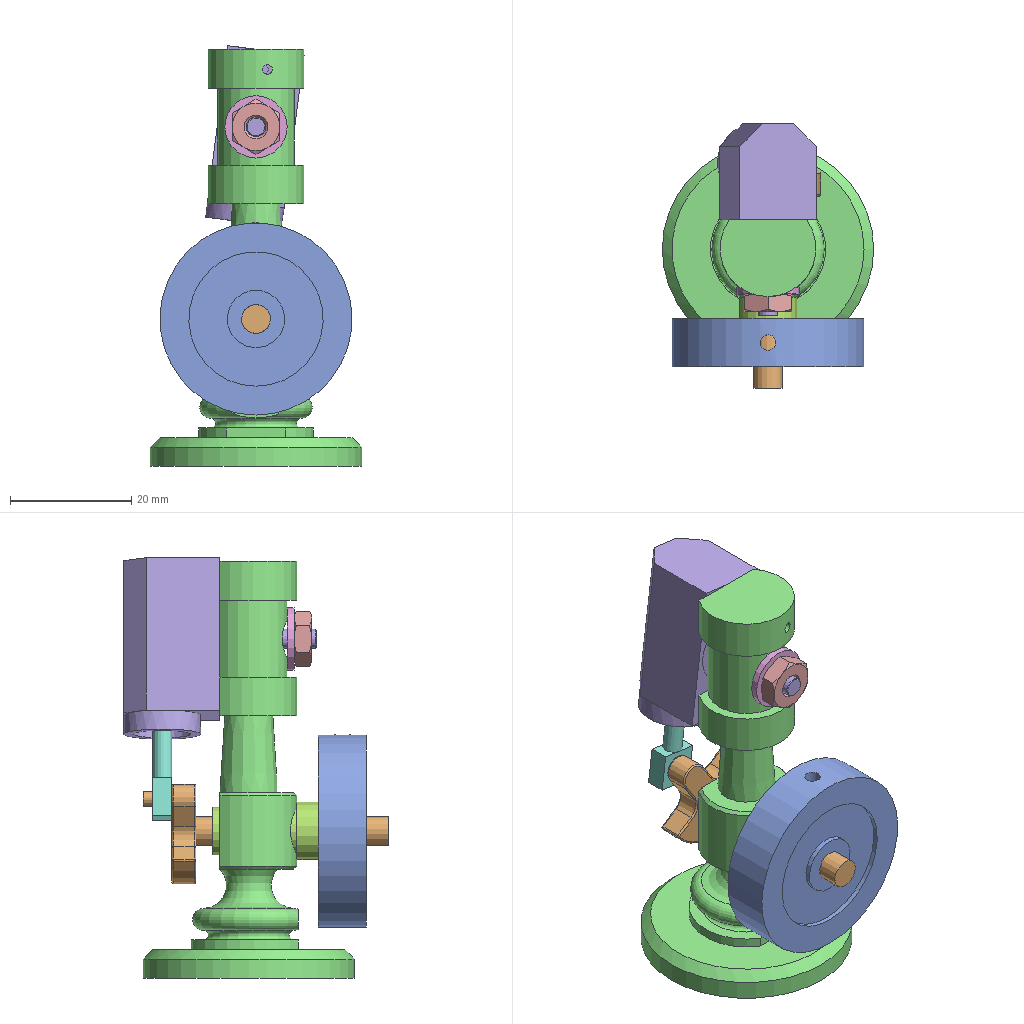Assembly | NX | 8 different items | 8 placed | box 35 x 44 x 70 mm
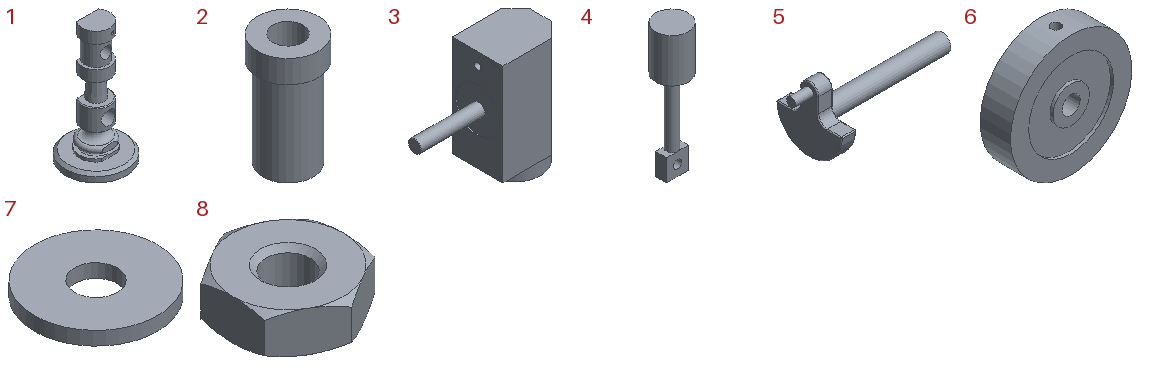Parts list (item | quantity | size | volume | features):
1 | x1 | 34.925 x 34.925 x 68.955 mm | 12101 mm3 | features DATUM_CSYS 9, SKETCH 8, EXTRUDE 5, CYLINDER 4, SWP104 3, CHAMFER 2, Intersection Curve 2, CPROJ 1
2 | x1 | 9.525 x 9.525 x 17.463 mm | 630.793 mm3 | features DATUM_CSYS 2, SKETCH 1, SWP104 1
3 | x1 | 31.75 x 12.7 x 28.575 mm | 3399 mm3 | features DATUM_CSYS 7, SKETCH 6, EXTRUDE 4, CYLINDER 2, CHAMFER 1, SWP104 1
4 | x1 | 9.525 x 9.525 x 38.1 mm | 1170 mm3 | features DATUM_CSYS 4, SKETCH 3, EXTRUDE 2, SWP104 1
5 | x1 | 40.481 x 17.455 x 17.462 mm | 1225 mm3 | features DATUM_CSYS 4, EXTRUDE 3, SKETCH 3, BLEND 1
6 | x1 | 31.75 x 7.938 x 31.75 mm | 5557 mm3 | features DATUM_CSYS 3, CYLINDER 2, SKETCH 2, DATUM_PLANE 1, SWP104 1
7 | x1 | 10.312 x 10.312 x 1.143 mm | 83.953 mm3 | features DATUM_CSYS 2, EXTRUDE 1, SKETCH 1
8 | x1 | 7.925 x 9.151 x 2.896 mm | 131.895 mm3 | features DATUM_CSYS 4, EXTRACT_DATUM_AXIS 4, SKETCH 3, EXTRACT_DATUM_PLANE 2, EXTRACT_FACE 2, EXTRACT_STRING 2, SWP104 2, CHAMFER 1, EXTRUDE 1, Instance Feature 1, Mirror Feature 1
Mates (type | each side: item.copy, entity, surface, feature):
Fix | 1.1 component
Touch | 3.1 face cylinder Tube(9) | 1.1 face cylinder Cylinder(11)
Touch | 3.1 face plane Extrude(2) | 1.1 face plane Extrude(7)
Touch | 4.1 face cylinder Revolve(3) | 3.1 face cylinder Cylinder(11)
Touch | 5.1 face cylinder Extrude(3) | 1.1 face cylinder Extrude(9)
Touch | 5.1 face cylinder Extrude(4) | 4.1 face cylinder Extrude(2)
Touch | 5.1 face plane Extrude(1) | 4.1 face plane Extrude(1)
Touch | 2.1 face cylinder Revolve(1) | 1.1 face cylinder Extrude(9)
Touch | 6.1 face cylinder Cylinder(2) | 5.1 face cylinder Extrude(3)
Touch | 2.1 face plane Revolve(1) | 1.1 face cylinder Revolve(6)
Touch | 6.1 face plane Revolve(1) | 2.1 face plane Revolve(1)
Touch | 7.1 face cylinder Extrude(1) | 3.1 face cylinder Tube(9)
Touch | 7.1 face plane Extrude(1) | 1.1 face cylinder Revolve(6)
Touch | 8.1 face cone Revolve(7) | 3.1 face cylinder Tube(9)
Touch | 8.1 face plane Extrude(1) | 7.1 face plane Extrude(1)